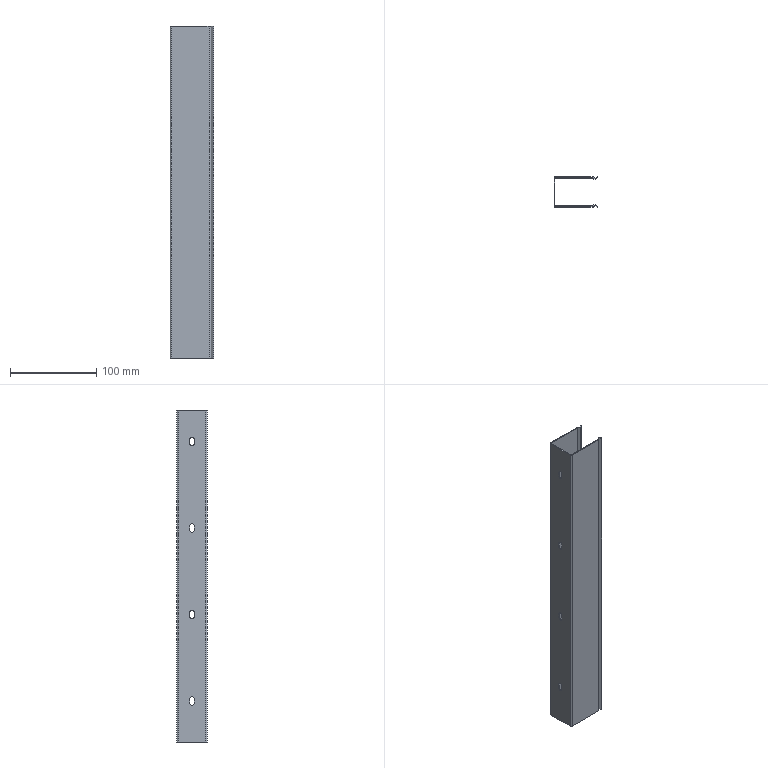Part | STEP file | 1 solid | 42 faces | box 50.625 x 35 x 384 mm | volume 51986 mm3 | plane 26 | cylinder 16 | commonest cylinder face diameters 5 x12 1 x2 3 x2